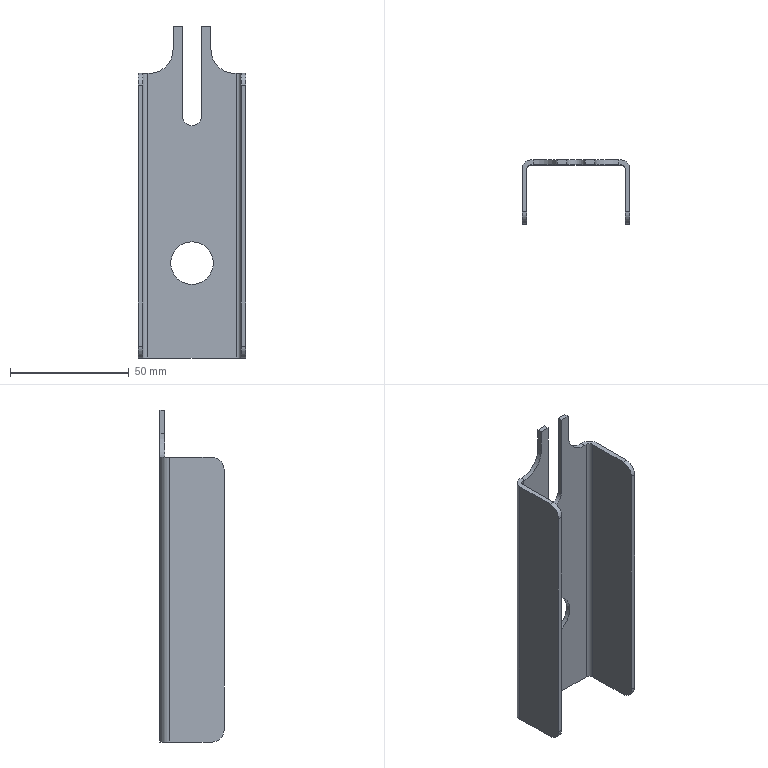Part | NX | features BREP 1 | 1 solid | 29 faces | box 45.5 x 27 x 140 mm | volume 21818 mm3 | plane 17 | cylinder 12 | commonest cylinder face diameters 10 x4 8 x3 4 x2 20 x2 18 x1
STEP:
#1=CARTESIAN_POINT('',(4.,0.,140.));
#2=VERTEX_POINT('',#1);
#3=CARTESIAN_POINT('',(4.,0.,102.));
#4=VERTEX_POINT('',#3);
#5=CARTESIAN_POINT('',(4.,0.,140.));
#6=DIRECTION('',(0.,0.,-1.));
#7=VECTOR('',#6,1000.);
#8=LINE('',#5,#7);
#9=EDGE_CURVE('',#2,#4,#8,.T.);
#10=ORIENTED_EDGE('',*,*,#9,.T.);
#11=CARTESIAN_POINT('',(-4.,0.,102.));
#12=VERTEX_POINT('',#11);
#13=CARTESIAN_POINT('',(0.,0.,102.));
#14=DIRECTION('',(0.,1.,0.));
#15=DIRECTION('',(0.,0.,1.));
#16=AXIS2_PLACEMENT_3D('',#13,#14,#15);
#17=CIRCLE('',#16,4.);
#18=EDGE_CURVE('',#4,#12,#17,.T.);
#19=ORIENTED_EDGE('',*,*,#18,.T.);
#20=CARTESIAN_POINT('',(-4.,0.,140.));
#21=VERTEX_POINT('',#20);
#22=CARTESIAN_POINT('',(-4.,0.,140.));
#23=DIRECTION('',(0.,0.,1.));
#24=VECTOR('',#23,1000.);
#25=LINE('',#22,#24);
#26=EDGE_CURVE('',#12,#21,#25,.T.);
#27=ORIENTED_EDGE('',*,*,#26,.T.);
#28=CARTESIAN_POINT('',(-8.,0.,140.));
#29=VERTEX_POINT('',#28);
#30=CARTESIAN_POINT('',(-20.75,0.,140.));
#31=DIRECTION('',(-1.,0.,0.));
#32=VECTOR('',#31,1000.);
#33=LINE('',#30,#32);
#34=EDGE_CURVE('',#21,#29,#33,.T.);
#35=ORIENTED_EDGE('',*,*,#34,.T.);
#36=CARTESIAN_POINT('',(-8.,0.,130.));
#37=VERTEX_POINT('',#36);
#38=CARTESIAN_POINT('',(-8.,0.,140.));
#39=DIRECTION('',(0.,0.,-1.));
#40=VECTOR('',#39,1000.);
#41=LINE('',#38,#40);
#42=EDGE_CURVE('',#29,#37,#41,.T.);
#43=ORIENTED_EDGE('',*,*,#42,.T.);
#44=CARTESIAN_POINT('',(-18.,0.,120.));
#45=VERTEX_POINT('',#44);
#46=CARTESIAN_POINT('',(-18.,0.,130.));
#47=DIRECTION('',(0.,1.,0.));
#48=DIRECTION('',(0.,0.,-1.));
#49=AXIS2_PLACEMENT_3D('',#46,#47,#48);
#50=CIRCLE('',#49,10.);
#51=EDGE_CURVE('',#37,#45,#50,.T.);
#52=ORIENTED_EDGE('',*,*,#51,.T.);
#53=CARTESIAN_POINT('',(-18.75,0.,120.));
#54=VERTEX_POINT('',#53);
#55=CARTESIAN_POINT('',(-8.,0.,120.));
#56=DIRECTION('',(-1.,0.,0.));
#57=VECTOR('',#56,1000.);
#58=LINE('',#55,#57);
#59=EDGE_CURVE('',#45,#54,#58,.T.);
#60=ORIENTED_EDGE('',*,*,#59,.T.);
#61=CARTESIAN_POINT('',(-18.75,0.,0.));
#62=VERTEX_POINT('',#61);
#63=CARTESIAN_POINT('',(-18.75,0.,140.));
#64=DIRECTION('',(0.,0.,-1.));
#65=VECTOR('',#64,1000.);
#66=LINE('',#63,#65);
#67=EDGE_CURVE('',#54,#62,#66,.T.);
#68=ORIENTED_EDGE('',*,*,#67,.T.);
#69=CARTESIAN_POINT('',(18.75,0.,0.));
#70=VERTEX_POINT('',#69);
#71=CARTESIAN_POINT('',(-20.75,0.,0.));
#72=DIRECTION('',(1.,0.,0.));
#73=VECTOR('',#72,1000.);
#74=LINE('',#71,#73);
#75=EDGE_CURVE('',#62,#70,#74,.T.);
#76=ORIENTED_EDGE('',*,*,#75,.T.);
#77=CARTESIAN_POINT('',(18.75,0.,120.));
#78=VERTEX_POINT('',#77);
#79=CARTESIAN_POINT('',(18.75,0.,140.));
#80=DIRECTION('',(0.,0.,1.));
#81=VECTOR('',#80,1000.);
#82=LINE('',#79,#81);
#83=EDGE_CURVE('',#70,#78,#82,.T.);
#84=ORIENTED_EDGE('',*,*,#83,.T.);
#85=CARTESIAN_POINT('',(18.,0.,120.));
#86=VERTEX_POINT('',#85);
#87=CARTESIAN_POINT('',(8.,0.,120.));
#88=DIRECTION('',(1.,0.,0.));
#89=VECTOR('',#88,1000.);
#90=LINE('',#87,#89);
#91=EDGE_CURVE('',#86,#78,#90,.T.);
#92=ORIENTED_EDGE('',*,*,#91,.F.);
#93=CARTESIAN_POINT('',(8.,0.,130.));
#94=VERTEX_POINT('',#93);
#95=CARTESIAN_POINT('',(18.,0.,130.));
#96=DIRECTION('',(0.,1.,0.));
#97=DIRECTION('',(0.,0.,-1.));
#98=AXIS2_PLACEMENT_3D('',#95,#96,#97);
#99=CIRCLE('',#98,10.);
#100=EDGE_CURVE('',#86,#94,#99,.T.);
#101=ORIENTED_EDGE('',*,*,#100,.T.);
#102=CARTESIAN_POINT('',(8.,0.,140.));
#103=VERTEX_POINT('',#102);
#104=CARTESIAN_POINT('',(8.,0.,140.));
#105=DIRECTION('',(0.,0.,1.));
#106=VECTOR('',#105,1000.);
#107=LINE('',#104,#106);
#108=EDGE_CURVE('',#94,#103,#107,.T.);
#109=ORIENTED_EDGE('',*,*,#108,.T.);
#110=CARTESIAN_POINT('',(-20.75,0.,140.));
#111=DIRECTION('',(-1.,0.,0.));
#112=VECTOR('',#111,1000.);
#113=LINE('',#110,#112);
#114=EDGE_CURVE('',#103,#2,#113,.T.);
#115=ORIENTED_EDGE('',*,*,#114,.T.);
#116=EDGE_LOOP('',(#10,#19,#27,#35,#43,#52,#60,#68,#76,#84,#92,#101,#109,#115));
#117=FACE_BOUND('',#116,.T.);
#118=CARTESIAN_POINT('',(0.,0.,49.));
#119=VERTEX_POINT('',#118);
#120=CARTESIAN_POINT('',(0.,0.,40.));
#121=DIRECTION('',(0.,1.,0.));
#122=DIRECTION('',(0.,0.,1.));
#123=AXIS2_PLACEMENT_3D('',#120,#121,#122);
#124=CIRCLE('',#123,9.);
#125=EDGE_CURVE('',#119,#119,#124,.T.);
#126=ORIENTED_EDGE('',*,*,#125,.T.);
#127=EDGE_LOOP('',(#126));
#128=FACE_BOUND('',#127,.T.);
#129=CARTESIAN_POINT('',(-20.75,0.,140.));
#130=DIRECTION('',(0.,-1.,0.));
#131=DIRECTION('',(0.,0.,1.));
#132=AXIS2_PLACEMENT_3D('',#129,#130,#131);
#133=PLANE('',#132);
#134=ADVANCED_FACE('',(#117,#128),#133,.T.);
#135=CARTESIAN_POINT('',(4.,2.,102.));
#136=VERTEX_POINT('',#135);
#137=CARTESIAN_POINT('',(4.,-8.,102.));
#138=DIRECTION('',(0.,-1.,0.));
#139=VECTOR('',#138,1000.);
#140=LINE('',#137,#139);
#141=EDGE_CURVE('',#136,#4,#140,.T.);
#142=ORIENTED_EDGE('',*,*,#141,.F.);
#143=CARTESIAN_POINT('',(-4.,2.,102.));
#144=VERTEX_POINT('',#143);
#145=CARTESIAN_POINT('',(0.,2.,102.));
#146=DIRECTION('',(0.,-1.,0.));
#147=DIRECTION('',(0.,0.,1.));
#148=AXIS2_PLACEMENT_3D('',#145,#146,#147);
#149=CIRCLE('',#148,4.);
#150=EDGE_CURVE('',#144,#136,#149,.T.);
#151=ORIENTED_EDGE('',*,*,#150,.F.);
#152=CARTESIAN_POINT('',(-4.,-8.,102.));
#153=DIRECTION('',(0.,1.,0.));
#154=VECTOR('',#153,1000.);
#155=LINE('',#152,#154);
#156=EDGE_CURVE('',#12,#144,#155,.T.);
#157=ORIENTED_EDGE('',*,*,#156,.F.);
#158=ORIENTED_EDGE('',*,*,#18,.F.);
#159=EDGE_LOOP('',(#142,#151,#157,#158));
#160=FACE_BOUND('',#159,.T.);
#161=CARTESIAN_POINT('',(0.,-8.,102.));
#162=DIRECTION('',(0.,1.,0.));
#163=DIRECTION('',(0.,0.,-1.));
#164=AXIS2_PLACEMENT_3D('',#161,#162,#163);
#165=CYLINDRICAL_SURFACE('',#164,4.);
#166=ADVANCED_FACE('',(#160),#165,.F.);
#167=CARTESIAN_POINT('',(4.,2.,140.));
#168=VERTEX_POINT('',#167);
#169=CARTESIAN_POINT('',(4.,-8.,140.));
#170=DIRECTION('',(0.,-1.,0.));
#171=VECTOR('',#170,1000.);
#172=LINE('',#169,#171);
#173=EDGE_CURVE('',#168,#2,#172,.T.);
#174=ORIENTED_EDGE('',*,*,#173,.F.);
#175=CARTESIAN_POINT('',(4.,2.,140.));
#176=DIRECTION('',(0.,0.,1.));
#177=VECTOR('',#176,1000.);
#178=LINE('',#175,#177);
#179=EDGE_CURVE('',#136,#168,#178,.T.);
#180=ORIENTED_EDGE('',*,*,#179,.F.);
#181=ORIENTED_EDGE('',*,*,#141,.T.);
#182=ORIENTED_EDGE('',*,*,#9,.F.);
#183=EDGE_LOOP('',(#174,#180,#181,#182));
#184=FACE_BOUND('',#183,.T.);
#185=CARTESIAN_POINT('',(4.,-8.,140.));
#186=DIRECTION('',(1.,0.,0.));
#187=DIRECTION('',(0.,0.,1.));
#188=AXIS2_PLACEMENT_3D('',#185,#186,#187);
#189=PLANE('',#188);
#190=ADVANCED_FACE('',(#184),#189,.F.);
#191=CARTESIAN_POINT('',(8.,2.,140.));
#192=VERTEX_POINT('',#191);
#193=CARTESIAN_POINT('',(8.,-2.,140.));
#194=DIRECTION('',(0.,1.,0.));
#195=VECTOR('',#194,1000.);
#196=LINE('',#193,#195);
#197=EDGE_CURVE('',#103,#192,#196,.T.);
#198=ORIENTED_EDGE('',*,*,#197,.T.);
#199=CARTESIAN_POINT('',(22.75,2.,140.));
#200=DIRECTION('',(-1.,0.,0.));
#201=VECTOR('',#200,1000.);
#202=LINE('',#199,#201);
#203=EDGE_CURVE('',#192,#168,#202,.T.);
#204=ORIENTED_EDGE('',*,*,#203,.T.);
#205=ORIENTED_EDGE('',*,*,#173,.T.);
#206=ORIENTED_EDGE('',*,*,#114,.F.);
#207=EDGE_LOOP('',(#198,#204,#205,#206));
#208=FACE_BOUND('',#207,.T.);
#209=CARTESIAN_POINT('',(22.75,-2.,140.));
#210=DIRECTION('',(0.,0.,1.));
#211=DIRECTION('',(-1.,0.,0.));
#212=AXIS2_PLACEMENT_3D('',#209,#210,#211);
#213=PLANE('',#212);
#214=ADVANCED_FACE('',(#208),#213,.T.);
#215=CARTESIAN_POINT('',(8.,2.,130.));
#216=VERTEX_POINT('',#215);
#217=CARTESIAN_POINT('',(8.,2.,120.));
#218=DIRECTION('',(0.,0.,1.));
#219=VECTOR('',#218,1000.);
#220=LINE('',#217,#219);
#221=EDGE_CURVE('',#216,#192,#220,.T.);
#222=ORIENTED_EDGE('',*,*,#221,.T.);
#223=ORIENTED_EDGE('',*,*,#197,.F.);
#224=ORIENTED_EDGE('',*,*,#108,.F.);
#225=CARTESIAN_POINT('',(8.,-25.,130.));
#226=DIRECTION('',(0.,1.,0.));
#227=VECTOR('',#226,1000.);
#228=LINE('',#225,#227);
#229=EDGE_CURVE('',#94,#216,#228,.T.);
#230=ORIENTED_EDGE('',*,*,#229,.T.);
#231=EDGE_LOOP('',(#222,#223,#224,#230));
#232=FACE_BOUND('',#231,.T.);
#233=CARTESIAN_POINT('',(8.,-25.,120.));
#234=DIRECTION('',(1.,0.,0.));
#235=DIRECTION('',(0.,0.,1.));
#236=AXIS2_PLACEMENT_3D('',#233,#234,#235);
#237=PLANE('',#236);
#238=ADVANCED_FACE('',(#232),#237,.T.);
#239=CARTESIAN_POINT('',(18.,2.,120.));
#240=VERTEX_POINT('',#239);
#241=CARTESIAN_POINT('',(18.,-25.,120.));
#242=DIRECTION('',(0.,-1.,0.));
#243=VECTOR('',#242,1000.);
#244=LINE('',#241,#243);
#245=EDGE_CURVE('',#240,#86,#244,.T.);
#246=ORIENTED_EDGE('',*,*,#245,.F.);
#247=CARTESIAN_POINT('',(18.,2.,130.));
#248=DIRECTION('',(0.,-1.,0.));
#249=DIRECTION('',(0.,0.,-1.));
#250=AXIS2_PLACEMENT_3D('',#247,#248,#249);
#251=CIRCLE('',#250,10.);
#252=EDGE_CURVE('',#216,#240,#251,.T.);
#253=ORIENTED_EDGE('',*,*,#252,.F.);
#254=ORIENTED_EDGE('',*,*,#229,.F.);
#255=ORIENTED_EDGE('',*,*,#100,.F.);
#256=EDGE_LOOP('',(#246,#253,#254,#255));
#257=FACE_BOUND('',#256,.T.);
#258=CARTESIAN_POINT('',(18.,-25.,130.));
#259=DIRECTION('',(0.,-1.,0.));
#260=DIRECTION('',(0.,0.,1.));
#261=AXIS2_PLACEMENT_3D('',#258,#259,#260);
#262=CYLINDRICAL_SURFACE('',#261,10.);
#263=ADVANCED_FACE('',(#257),#262,.F.);
#264=CARTESIAN_POINT('',(20.75,-2.,120.));
#265=VERTEX_POINT('',#264);
#266=CARTESIAN_POINT('',(18.75,-2.,120.));
#267=DIRECTION('',(0.,0.,-1.));
#268=DIRECTION('',(-1.,0.,0.));
#269=AXIS2_PLACEMENT_3D('',#266,#267,#268);
#270=CIRCLE('',#269,2.);
#271=EDGE_CURVE('',#78,#265,#270,.T.);
#272=ORIENTED_EDGE('',*,*,#271,.F.);
#273=ORIENTED_EDGE('',*,*,#83,.F.);
#274=CARTESIAN_POINT('',(20.75,-2.,0.));
#275=VERTEX_POINT('',#274);
#276=CARTESIAN_POINT('',(18.75,-2.,0.));
#277=DIRECTION('',(0.,0.,1.));
#278=DIRECTION('',(-1.,0.,0.));
#279=AXIS2_PLACEMENT_3D('',#276,#277,#278);
#280=CIRCLE('',#279,2.);
#281=EDGE_CURVE('',#275,#70,#280,.T.);
#282=ORIENTED_EDGE('',*,*,#281,.F.);
#283=CARTESIAN_POINT('',(20.75,-2.,140.));
#284=DIRECTION('',(0.,0.,-1.));
#285=VECTOR('',#284,1000.);
#286=LINE('',#283,#285);
#287=EDGE_CURVE('',#265,#275,#286,.T.);
#288=ORIENTED_EDGE('',*,*,#287,.F.);
#289=EDGE_LOOP('',(#272,#273,#282,#288));
#290=FACE_BOUND('',#289,.T.);
#291=CARTESIAN_POINT('',(18.75,-2.,140.));
#292=DIRECTION('',(0.,0.,-1.));
#293=DIRECTION('',(1.,0.,0.));
#294=AXIS2_PLACEMENT_3D('',#291,#292,#293);
#295=CYLINDRICAL_SURFACE('',#294,2.);
#296=ADVANCED_FACE('',(#290),#295,.F.);
#297=CARTESIAN_POINT('',(-18.75,2.,0.));
#298=VERTEX_POINT('',#297);
#299=CARTESIAN_POINT('',(18.75,2.,0.));
#300=VERTEX_POINT('',#299);
#301=CARTESIAN_POINT('',(-22.75,2.,0.));
#302=DIRECTION('',(1.,0.,0.));
#303=VECTOR('',#302,1000.);
#304=LINE('',#301,#303);
#305=EDGE_CURVE('',#298,#300,#304,.T.);
#306=ORIENTED_EDGE('',*,*,#305,.T.);
#307=CARTESIAN_POINT('',(22.75,-2.,0.));
#308=VERTEX_POINT('',#307);
#309=CARTESIAN_POINT('',(18.75,-2.,0.));
#310=DIRECTION('',(0.,0.,-1.));
#311=DIRECTION('',(-1.,0.,0.));
#312=AXIS2_PLACEMENT_3D('',#309,#310,#311);
#313=CIRCLE('',#312,4.);
#314=EDGE_CURVE('',#300,#308,#313,.T.);
#315=ORIENTED_EDGE('',*,*,#314,.T.);
#316=CARTESIAN_POINT('',(22.75,-20.,0.));
#317=VERTEX_POINT('',#316);
#318=CARTESIAN_POINT('',(22.75,0.,0.));
#319=DIRECTION('',(0.,-1.,0.));
#320=VECTOR('',#319,1000.);
#321=LINE('',#318,#320);
#322=EDGE_CURVE('',#308,#317,#321,.T.);
#323=ORIENTED_EDGE('',*,*,#322,.T.);
#324=CARTESIAN_POINT('',(20.75,-20.,0.));
#325=VERTEX_POINT('',#324);
#326=CARTESIAN_POINT('',(18.75,-20.,0.));
#327=DIRECTION('',(1.,0.,0.));
#328=VECTOR('',#327,1000.);
#329=LINE('',#326,#328);
#330=EDGE_CURVE('',#325,#317,#329,.T.);
#331=ORIENTED_EDGE('',*,*,#330,.F.);
#332=CARTESIAN_POINT('',(20.75,0.,0.));
#333=DIRECTION('',(0.,-1.,0.));
#334=VECTOR('',#333,1000.);
#335=LINE('',#332,#334);
#336=EDGE_CURVE('',#275,#325,#335,.T.);
#337=ORIENTED_EDGE('',*,*,#336,.F.);
#338=ORIENTED_EDGE('',*,*,#281,.T.);
#339=ORIENTED_EDGE('',*,*,#75,.F.);
#340=CARTESIAN_POINT('',(-20.75,-2.,0.));
#341=VERTEX_POINT('',#340);
#342=CARTESIAN_POINT('',(-18.75,-2.,0.));
#343=DIRECTION('',(0.,0.,1.));
#344=DIRECTION('',(-1.,0.,0.));
#345=AXIS2_PLACEMENT_3D('',#342,#343,#344);
#346=CIRCLE('',#345,2.);
#347=EDGE_CURVE('',#62,#341,#346,.T.);
#348=ORIENTED_EDGE('',*,*,#347,.T.);
#349=CARTESIAN_POINT('',(-20.75,-20.,0.));
#350=VERTEX_POINT('',#349);
#351=CARTESIAN_POINT('',(-20.75,0.,0.));
#352=DIRECTION('',(0.,1.,0.));
#353=VECTOR('',#352,1000.);
#354=LINE('',#351,#353);
#355=EDGE_CURVE('',#350,#341,#354,.T.);
#356=ORIENTED_EDGE('',*,*,#355,.F.);
#357=CARTESIAN_POINT('',(-22.75,-20.,0.));
#358=VERTEX_POINT('',#357);
#359=CARTESIAN_POINT('',(-18.75,-20.,0.));
#360=DIRECTION('',(-1.,0.,0.));
#361=VECTOR('',#360,1000.);
#362=LINE('',#359,#361);
#363=EDGE_CURVE('',#350,#358,#362,.T.);
#364=ORIENTED_EDGE('',*,*,#363,.T.);
#365=CARTESIAN_POINT('',(-22.75,-2.,0.));
#366=VERTEX_POINT('',#365);
#367=CARTESIAN_POINT('',(-22.75,-2.,0.));
#368=DIRECTION('',(0.,1.,0.));
#369=VECTOR('',#368,1000.);
#370=LINE('',#367,#369);
#371=EDGE_CURVE('',#358,#366,#370,.T.);
#372=ORIENTED_EDGE('',*,*,#371,.T.);
#373=CARTESIAN_POINT('',(-18.75,-2.,0.));
#374=DIRECTION('',(0.,0.,-1.));
#375=DIRECTION('',(-1.,0.,0.));
#376=AXIS2_PLACEMENT_3D('',#373,#374,#375);
#377=CIRCLE('',#376,4.);
#378=EDGE_CURVE('',#366,#298,#377,.T.);
#379=ORIENTED_EDGE('',*,*,#378,.T.);
#380=EDGE_LOOP('',(#306,#315,#323,#331,#337,#338,#339,#348,#356,#364,#372,#379));
#381=FACE_BOUND('',#380,.T.);
#382=CARTESIAN_POINT('',(-22.75,-2.,0.));
#383=DIRECTION('',(0.,0.,-1.));
#384=DIRECTION('',(1.,0.,0.));
#385=AXIS2_PLACEMENT_3D('',#382,#383,#384);
#386=PLANE('',#385);
#387=ADVANCED_FACE('',(#381),#386,.T.);
#388=CARTESIAN_POINT('',(-20.75,-2.,120.));
#389=VERTEX_POINT('',#388);
#390=CARTESIAN_POINT('',(-20.75,-2.,140.));
#391=DIRECTION('',(0.,0.,1.));
#392=VECTOR('',#391,1000.);
#393=LINE('',#390,#392);
#394=EDGE_CURVE('',#341,#389,#393,.T.);
#395=ORIENTED_EDGE('',*,*,#394,.F.);
#396=ORIENTED_EDGE('',*,*,#347,.F.);
#397=ORIENTED_EDGE('',*,*,#67,.F.);
#398=CARTESIAN_POINT('',(-18.75,-2.,120.));
#399=DIRECTION('',(0.,0.,-1.));
#400=DIRECTION('',(-1.,0.,0.));
#401=AXIS2_PLACEMENT_3D('',#398,#399,#400);
#402=CIRCLE('',#401,2.);
#403=EDGE_CURVE('',#389,#54,#402,.T.);
#404=ORIENTED_EDGE('',*,*,#403,.F.);
#405=EDGE_LOOP('',(#395,#396,#397,#404));
#406=FACE_BOUND('',#405,.T.);
#407=CARTESIAN_POINT('',(-18.75,-2.,140.));
#408=DIRECTION('',(0.,0.,-1.));
#409=DIRECTION('',(1.,0.,0.));
#410=AXIS2_PLACEMENT_3D('',#407,#408,#409);
#411=CYLINDRICAL_SURFACE('',#410,2.);
#412=ADVANCED_FACE('',(#406),#411,.F.);
#413=CARTESIAN_POINT('',(-8.,2.,130.));
#414=VERTEX_POINT('',#413);
#415=CARTESIAN_POINT('',(-8.,-25.,130.));
#416=DIRECTION('',(0.,-1.,0.));
#417=VECTOR('',#416,1000.);
#418=LINE('',#415,#417);
#419=EDGE_CURVE('',#414,#37,#418,.T.);
#420=ORIENTED_EDGE('',*,*,#419,.F.);
#421=CARTESIAN_POINT('',(-18.,2.,120.));
#422=VERTEX_POINT('',#421);
#423=CARTESIAN_POINT('',(-18.,2.,130.));
#424=DIRECTION('',(0.,-1.,0.));
#425=DIRECTION('',(0.,0.,-1.));
#426=AXIS2_PLACEMENT_3D('',#423,#424,#425);
#427=CIRCLE('',#426,10.);
#428=EDGE_CURVE('',#422,#414,#427,.T.);
#429=ORIENTED_EDGE('',*,*,#428,.F.);
#430=CARTESIAN_POINT('',(-18.,-25.,120.));
#431=DIRECTION('',(0.,1.,0.));
#432=VECTOR('',#431,1000.);
#433=LINE('',#430,#432);
#434=EDGE_CURVE('',#45,#422,#433,.T.);
#435=ORIENTED_EDGE('',*,*,#434,.F.);
#436=ORIENTED_EDGE('',*,*,#51,.F.);
#437=EDGE_LOOP('',(#420,#429,#435,#436));
#438=FACE_BOUND('',#437,.T.);
#439=CARTESIAN_POINT('',(-18.,-25.,130.));
#440=DIRECTION('',(0.,-1.,0.));
#441=DIRECTION('',(0.,0.,1.));
#442=AXIS2_PLACEMENT_3D('',#439,#440,#441);
#443=CYLINDRICAL_SURFACE('',#442,10.);
#444=ADVANCED_FACE('',(#438),#443,.F.);
#445=ORIENTED_EDGE('',*,*,#419,.T.);
#446=ORIENTED_EDGE('',*,*,#42,.F.);
#447=CARTESIAN_POINT('',(-8.,2.,140.));
#448=VERTEX_POINT('',#447);
#449=CARTESIAN_POINT('',(-8.,-25.,140.));
#450=DIRECTION('',(0.,-1.,0.));
#451=VECTOR('',#450,1000.);
#452=LINE('',#449,#451);
#453=EDGE_CURVE('',#448,#29,#452,.T.);
#454=ORIENTED_EDGE('',*,*,#453,.F.);
#455=CARTESIAN_POINT('',(-8.,2.,120.));
#456=DIRECTION('',(0.,0.,1.));
#457=VECTOR('',#456,1000.);
#458=LINE('',#455,#457);
#459=EDGE_CURVE('',#414,#448,#458,.T.);
#460=ORIENTED_EDGE('',*,*,#459,.F.);
#461=EDGE_LOOP('',(#445,#446,#454,#460));
#462=FACE_BOUND('',#461,.T.);
#463=CARTESIAN_POINT('',(-8.,-25.,120.));
#464=DIRECTION('',(1.,0.,0.));
#465=DIRECTION('',(0.,0.,1.));
#466=AXIS2_PLACEMENT_3D('',#463,#464,#465);
#467=PLANE('',#466);
#468=ADVANCED_FACE('',(#462),#467,.F.);
#469=ORIENTED_EDGE('',*,*,#453,.T.);
#470=ORIENTED_EDGE('',*,*,#34,.F.);
#471=CARTESIAN_POINT('',(-4.,2.,140.));
#472=VERTEX_POINT('',#471);
#473=CARTESIAN_POINT('',(-4.,-2.,140.));
#474=DIRECTION('',(0.,1.,0.));
#475=VECTOR('',#474,1000.);
#476=LINE('',#473,#475);
#477=EDGE_CURVE('',#21,#472,#476,.T.);
#478=ORIENTED_EDGE('',*,*,#477,.T.);
#479=CARTESIAN_POINT('',(22.75,2.,140.));
#480=DIRECTION('',(-1.,0.,0.));
#481=VECTOR('',#480,1000.);
#482=LINE('',#479,#481);
#483=EDGE_CURVE('',#472,#448,#482,.T.);
#484=ORIENTED_EDGE('',*,*,#483,.T.);
#485=EDGE_LOOP('',(#469,#470,#478,#484));
#486=FACE_BOUND('',#485,.T.);
#487=CARTESIAN_POINT('',(22.75,-2.,140.));
#488=DIRECTION('',(0.,0.,1.));
#489=DIRECTION('',(-1.,0.,0.));
#490=AXIS2_PLACEMENT_3D('',#487,#488,#489);
#491=PLANE('',#490);
#492=ADVANCED_FACE('',(#486),#491,.T.);
#493=ORIENTED_EDGE('',*,*,#156,.T.);
#494=CARTESIAN_POINT('',(-4.,2.,140.));
#495=DIRECTION('',(0.,0.,-1.));
#496=VECTOR('',#495,1000.);
#497=LINE('',#494,#496);
#498=EDGE_CURVE('',#472,#144,#497,.T.);
#499=ORIENTED_EDGE('',*,*,#498,.F.);
#500=ORIENTED_EDGE('',*,*,#477,.F.);
#501=ORIENTED_EDGE('',*,*,#26,.F.);
#502=EDGE_LOOP('',(#493,#499,#500,#501));
#503=FACE_BOUND('',#502,.T.);
#504=CARTESIAN_POINT('',(-4.,-8.,140.));
#505=DIRECTION('',(-1.,0.,0.));
#506=DIRECTION('',(0.,0.,-1.));
#507=AXIS2_PLACEMENT_3D('',#504,#505,#506);
#508=PLANE('',#507);
#509=ADVANCED_FACE('',(#503),#508,.F.);
#510=ORIENTED_EDGE('',*,*,#125,.F.);
#511=EDGE_LOOP('',(#510));
#512=FACE_BOUND('',#511,.T.);
#513=CARTESIAN_POINT('',(0.,2.,49.));
#514=VERTEX_POINT('',#513);
#515=CARTESIAN_POINT('',(0.,2.,40.));
#516=DIRECTION('',(0.,-1.,0.));
#517=DIRECTION('',(0.,0.,1.));
#518=AXIS2_PLACEMENT_3D('',#515,#516,#517);
#519=CIRCLE('',#518,9.);
#520=EDGE_CURVE('',#514,#514,#519,.T.);
#521=ORIENTED_EDGE('',*,*,#520,.F.);
#522=EDGE_LOOP('',(#521));
#523=FACE_BOUND('',#522,.T.);
#524=CARTESIAN_POINT('',(0.,-8.,40.));
#525=DIRECTION('',(0.,1.,0.));
#526=DIRECTION('',(0.,0.,-1.));
#527=AXIS2_PLACEMENT_3D('',#524,#525,#526);
#528=CYLINDRICAL_SURFACE('',#527,9.);
#529=ADVANCED_FACE('',(#512,#523),#528,.F.);
#530=ORIENTED_EDGE('',*,*,#498,.T.);
#531=ORIENTED_EDGE('',*,*,#150,.T.);
#532=ORIENTED_EDGE('',*,*,#179,.T.);
#533=ORIENTED_EDGE('',*,*,#203,.F.);
#534=ORIENTED_EDGE('',*,*,#221,.F.);
#535=ORIENTED_EDGE('',*,*,#252,.T.);
#536=CARTESIAN_POINT('',(18.75,2.,120.));
#537=VERTEX_POINT('',#536);
#538=CARTESIAN_POINT('',(-20.75,2.,120.));
#539=DIRECTION('',(-1.,0.,0.));
#540=VECTOR('',#539,1000.);
#541=LINE('',#538,#540);
#542=EDGE_CURVE('',#537,#240,#541,.T.);
#543=ORIENTED_EDGE('',*,*,#542,.F.);
#544=CARTESIAN_POINT('',(18.75,2.,140.));
#545=DIRECTION('',(0.,0.,1.));
#546=VECTOR('',#545,1000.);
#547=LINE('',#544,#546);
#548=EDGE_CURVE('',#300,#537,#547,.T.);
#549=ORIENTED_EDGE('',*,*,#548,.F.);
#550=ORIENTED_EDGE('',*,*,#305,.F.);
#551=CARTESIAN_POINT('',(-18.75,2.,120.));
#552=VERTEX_POINT('',#551);
#553=CARTESIAN_POINT('',(-18.75,2.,140.));
#554=DIRECTION('',(0.,0.,-1.));
#555=VECTOR('',#554,1000.);
#556=LINE('',#553,#555);
#557=EDGE_CURVE('',#552,#298,#556,.T.);
#558=ORIENTED_EDGE('',*,*,#557,.F.);
#559=CARTESIAN_POINT('',(-20.75,2.,120.));
#560=DIRECTION('',(-1.,0.,0.));
#561=VECTOR('',#560,1000.);
#562=LINE('',#559,#561);
#563=EDGE_CURVE('',#422,#552,#562,.T.);
#564=ORIENTED_EDGE('',*,*,#563,.F.);
#565=ORIENTED_EDGE('',*,*,#428,.T.);
#566=ORIENTED_EDGE('',*,*,#459,.T.);
#567=ORIENTED_EDGE('',*,*,#483,.F.);
#568=EDGE_LOOP('',(#530,#531,#532,#533,#534,#535,#543,#549,#550,#558,#564,#565,#566,#567));
#569=FACE_BOUND('',#568,.T.);
#570=ORIENTED_EDGE('',*,*,#520,.T.);
#571=EDGE_LOOP('',(#570));
#572=FACE_BOUND('',#571,.T.);
#573=CARTESIAN_POINT('',(-20.75,2.,140.));
#574=DIRECTION('',(0.,-1.,0.));
#575=DIRECTION('',(0.,0.,1.));
#576=AXIS2_PLACEMENT_3D('',#573,#574,#575);
#577=PLANE('',#576);
#578=ADVANCED_FACE('',(#569,#572),#577,.F.);
#579=ORIENTED_EDGE('',*,*,#91,.T.);
#580=ORIENTED_EDGE('',*,*,#271,.T.);
#581=CARTESIAN_POINT('',(20.75,-20.,120.));
#582=VERTEX_POINT('',#581);
#583=CARTESIAN_POINT('',(20.75,-25.,120.));
#584=DIRECTION('',(0.,-1.,0.));
#585=VECTOR('',#584,1000.);
#586=LINE('',#583,#585);
#587=EDGE_CURVE('',#265,#582,#586,.T.);
#588=ORIENTED_EDGE('',*,*,#587,.T.);
#589=CARTESIAN_POINT('',(22.75,-20.,120.));
#590=VERTEX_POINT('',#589);
#591=CARTESIAN_POINT('',(8.,-20.,120.));
#592=DIRECTION('',(1.,0.,0.));
#593=VECTOR('',#592,1000.);
#594=LINE('',#591,#593);
#595=EDGE_CURVE('',#582,#590,#594,.T.);
#596=ORIENTED_EDGE('',*,*,#595,.T.);
#597=CARTESIAN_POINT('',(22.75,-2.,120.));
#598=VERTEX_POINT('',#597);
#599=CARTESIAN_POINT('',(22.75,-25.,120.));
#600=DIRECTION('',(0.,1.,0.));
#601=VECTOR('',#600,1000.);
#602=LINE('',#599,#601);
#603=EDGE_CURVE('',#590,#598,#602,.T.);
#604=ORIENTED_EDGE('',*,*,#603,.T.);
#605=CARTESIAN_POINT('',(18.75,-2.,120.));
#606=DIRECTION('',(0.,0.,1.));
#607=DIRECTION('',(-1.,0.,0.));
#608=AXIS2_PLACEMENT_3D('',#605,#606,#607);
#609=CIRCLE('',#608,4.);
#610=EDGE_CURVE('',#598,#537,#609,.T.);
#611=ORIENTED_EDGE('',*,*,#610,.T.);
#612=ORIENTED_EDGE('',*,*,#542,.T.);
#613=ORIENTED_EDGE('',*,*,#245,.T.);
#614=EDGE_LOOP('',(#579,#580,#588,#596,#604,#611,#612,#613));
#615=FACE_BOUND('',#614,.T.);
#616=CARTESIAN_POINT('',(8.,-25.,120.));
#617=DIRECTION('',(0.,0.,1.));
#618=DIRECTION('',(-1.,0.,0.));
#619=AXIS2_PLACEMENT_3D('',#616,#617,#618);
#620=PLANE('',#619);
#621=ADVANCED_FACE('',(#615),#620,.T.);
#622=ORIENTED_EDGE('',*,*,#336,.T.);
#623=CARTESIAN_POINT('',(20.75,-25.,5.));
#624=VERTEX_POINT('',#623);
#625=CARTESIAN_POINT('',(20.75,-20.,5.));
#626=DIRECTION('',(-1.,0.,0.));
#627=DIRECTION('',(0.,0.,1.));
#628=AXIS2_PLACEMENT_3D('',#625,#626,#627);
#629=CIRCLE('',#628,5.);
#630=EDGE_CURVE('',#325,#624,#629,.T.);
#631=ORIENTED_EDGE('',*,*,#630,.T.);
#632=CARTESIAN_POINT('',(20.75,-25.,115.));
#633=VERTEX_POINT('',#632);
#634=CARTESIAN_POINT('',(20.75,-25.,140.));
#635=DIRECTION('',(0.,0.,1.));
#636=VECTOR('',#635,1000.);
#637=LINE('',#634,#636);
#638=EDGE_CURVE('',#624,#633,#637,.T.);
#639=ORIENTED_EDGE('',*,*,#638,.T.);
#640=CARTESIAN_POINT('',(20.75,-20.,115.));
#641=DIRECTION('',(-1.,0.,0.));
#642=DIRECTION('',(0.,0.,-1.));
#643=AXIS2_PLACEMENT_3D('',#640,#641,#642);
#644=CIRCLE('',#643,5.);
#645=EDGE_CURVE('',#633,#582,#644,.T.);
#646=ORIENTED_EDGE('',*,*,#645,.T.);
#647=ORIENTED_EDGE('',*,*,#587,.F.);
#648=ORIENTED_EDGE('',*,*,#287,.T.);
#649=EDGE_LOOP('',(#622,#631,#639,#646,#647,#648));
#650=FACE_BOUND('',#649,.T.);
#651=CARTESIAN_POINT('',(20.75,0.,140.));
#652=DIRECTION('',(-1.,0.,0.));
#653=DIRECTION('',(0.,0.,-1.));
#654=AXIS2_PLACEMENT_3D('',#651,#652,#653);
#655=PLANE('',#654);
#656=ADVANCED_FACE('',(#650),#655,.T.);
#657=CARTESIAN_POINT('',(-20.75,-20.,120.));
#658=VERTEX_POINT('',#657);
#659=CARTESIAN_POINT('',(-22.75,-20.,120.));
#660=VERTEX_POINT('',#659);
#661=CARTESIAN_POINT('',(-8.,-20.,120.));
#662=DIRECTION('',(-1.,0.,0.));
#663=VECTOR('',#662,1000.);
#664=LINE('',#661,#663);
#665=EDGE_CURVE('',#658,#660,#664,.T.);
#666=ORIENTED_EDGE('',*,*,#665,.F.);
#667=CARTESIAN_POINT('',(-20.75,-25.,120.));
#668=DIRECTION('',(0.,-1.,0.));
#669=VECTOR('',#668,1000.);
#670=LINE('',#667,#669);
#671=EDGE_CURVE('',#389,#658,#670,.T.);
#672=ORIENTED_EDGE('',*,*,#671,.F.);
#673=ORIENTED_EDGE('',*,*,#403,.T.);
#674=ORIENTED_EDGE('',*,*,#59,.F.);
#675=ORIENTED_EDGE('',*,*,#434,.T.);
#676=ORIENTED_EDGE('',*,*,#563,.T.);
#677=CARTESIAN_POINT('',(-22.75,-2.,120.));
#678=VERTEX_POINT('',#677);
#679=CARTESIAN_POINT('',(-18.75,-2.,120.));
#680=DIRECTION('',(0.,0.,-1.));
#681=DIRECTION('',(-1.,0.,0.));
#682=AXIS2_PLACEMENT_3D('',#679,#680,#681);
#683=CIRCLE('',#682,4.);
#684=EDGE_CURVE('',#678,#552,#683,.T.);
#685=ORIENTED_EDGE('',*,*,#684,.F.);
#686=CARTESIAN_POINT('',(-22.75,-25.,120.));
#687=DIRECTION('',(0.,1.,0.));
#688=VECTOR('',#687,1000.);
#689=LINE('',#686,#688);
#690=EDGE_CURVE('',#660,#678,#689,.T.);
#691=ORIENTED_EDGE('',*,*,#690,.F.);
#692=EDGE_LOOP('',(#666,#672,#673,#674,#675,#676,#685,#691));
#693=FACE_BOUND('',#692,.T.);
#694=CARTESIAN_POINT('',(-8.,-25.,120.));
#695=DIRECTION('',(0.,0.,-1.));
#696=DIRECTION('',(1.,0.,0.));
#697=AXIS2_PLACEMENT_3D('',#694,#695,#696);
#698=PLANE('',#697);
#699=ADVANCED_FACE('',(#693),#698,.F.);
#700=ORIENTED_EDGE('',*,*,#355,.T.);
#701=ORIENTED_EDGE('',*,*,#394,.T.);
#702=ORIENTED_EDGE('',*,*,#671,.T.);
#703=CARTESIAN_POINT('',(-20.75,-25.,115.));
#704=VERTEX_POINT('',#703);
#705=CARTESIAN_POINT('',(-20.75,-20.,115.));
#706=DIRECTION('',(1.,0.,0.));
#707=DIRECTION('',(0.,0.,-1.));
#708=AXIS2_PLACEMENT_3D('',#705,#706,#707);
#709=CIRCLE('',#708,5.);
#710=EDGE_CURVE('',#658,#704,#709,.T.);
#711=ORIENTED_EDGE('',*,*,#710,.T.);
#712=CARTESIAN_POINT('',(-20.75,-25.,5.));
#713=VERTEX_POINT('',#712);
#714=CARTESIAN_POINT('',(-20.75,-25.,140.));
#715=DIRECTION('',(0.,0.,-1.));
#716=VECTOR('',#715,1000.);
#717=LINE('',#714,#716);
#718=EDGE_CURVE('',#704,#713,#717,.T.);
#719=ORIENTED_EDGE('',*,*,#718,.T.);
#720=CARTESIAN_POINT('',(-20.75,-20.,5.));
#721=DIRECTION('',(1.,0.,0.));
#722=DIRECTION('',(0.,0.,1.));
#723=AXIS2_PLACEMENT_3D('',#720,#721,#722);
#724=CIRCLE('',#723,5.);
#725=EDGE_CURVE('',#713,#350,#724,.T.);
#726=ORIENTED_EDGE('',*,*,#725,.T.);
#727=EDGE_LOOP('',(#700,#701,#702,#711,#719,#726));
#728=FACE_BOUND('',#727,.T.);
#729=CARTESIAN_POINT('',(-20.75,0.,140.));
#730=DIRECTION('',(1.,0.,0.));
#731=DIRECTION('',(0.,0.,1.));
#732=AXIS2_PLACEMENT_3D('',#729,#730,#731);
#733=PLANE('',#732);
#734=ADVANCED_FACE('',(#728),#733,.T.);
#735=ORIENTED_EDGE('',*,*,#314,.F.);
#736=ORIENTED_EDGE('',*,*,#548,.T.);
#737=ORIENTED_EDGE('',*,*,#610,.F.);
#738=CARTESIAN_POINT('',(22.75,-2.,140.));
#739=DIRECTION('',(0.,0.,-1.));
#740=VECTOR('',#739,1000.);
#741=LINE('',#738,#740);
#742=EDGE_CURVE('',#598,#308,#741,.T.);
#743=ORIENTED_EDGE('',*,*,#742,.T.);
#744=EDGE_LOOP('',(#735,#736,#737,#743));
#745=FACE_BOUND('',#744,.T.);
#746=CARTESIAN_POINT('',(18.75,-2.,140.));
#747=DIRECTION('',(0.,0.,-1.));
#748=DIRECTION('',(1.,0.,0.));
#749=AXIS2_PLACEMENT_3D('',#746,#747,#748);
#750=CYLINDRICAL_SURFACE('',#749,4.);
#751=ADVANCED_FACE('',(#745),#750,.T.);
#752=ORIENTED_EDGE('',*,*,#557,.T.);
#753=ORIENTED_EDGE('',*,*,#378,.F.);
#754=CARTESIAN_POINT('',(-22.75,-2.,140.));
#755=DIRECTION('',(0.,0.,1.));
#756=VECTOR('',#755,1000.);
#757=LINE('',#754,#756);
#758=EDGE_CURVE('',#366,#678,#757,.T.);
#759=ORIENTED_EDGE('',*,*,#758,.T.);
#760=ORIENTED_EDGE('',*,*,#684,.T.);
#761=EDGE_LOOP('',(#752,#753,#759,#760));
#762=FACE_BOUND('',#761,.T.);
#763=CARTESIAN_POINT('',(-18.75,-2.,140.));
#764=DIRECTION('',(0.,0.,-1.));
#765=DIRECTION('',(1.,0.,0.));
#766=AXIS2_PLACEMENT_3D('',#763,#764,#765);
#767=CYLINDRICAL_SURFACE('',#766,4.);
#768=ADVANCED_FACE('',(#762),#767,.T.);
#769=CARTESIAN_POINT('',(22.75,-25.,115.));
#770=VERTEX_POINT('',#769);
#771=CARTESIAN_POINT('',(22.75,-20.,115.));
#772=DIRECTION('',(-1.,0.,0.));
#773=DIRECTION('',(0.,0.,-1.));
#774=AXIS2_PLACEMENT_3D('',#771,#772,#773);
#775=CIRCLE('',#774,5.);
#776=EDGE_CURVE('',#770,#590,#775,.T.);
#777=ORIENTED_EDGE('',*,*,#776,.F.);
#778=CARTESIAN_POINT('',(22.75,-25.,5.));
#779=VERTEX_POINT('',#778);
#780=CARTESIAN_POINT('',(22.75,-25.,140.));
#781=DIRECTION('',(0.,0.,1.));
#782=VECTOR('',#781,1000.);
#783=LINE('',#780,#782);
#784=EDGE_CURVE('',#779,#770,#783,.T.);
#785=ORIENTED_EDGE('',*,*,#784,.F.);
#786=CARTESIAN_POINT('',(22.75,-20.,5.));
#787=DIRECTION('',(-1.,0.,0.));
#788=DIRECTION('',(0.,0.,1.));
#789=AXIS2_PLACEMENT_3D('',#786,#787,#788);
#790=CIRCLE('',#789,5.);
#791=EDGE_CURVE('',#317,#779,#790,.T.);
#792=ORIENTED_EDGE('',*,*,#791,.F.);
#793=ORIENTED_EDGE('',*,*,#322,.F.);
#794=ORIENTED_EDGE('',*,*,#742,.F.);
#795=ORIENTED_EDGE('',*,*,#603,.F.);
#796=EDGE_LOOP('',(#777,#785,#792,#793,#794,#795));
#797=FACE_BOUND('',#796,.T.);
#798=CARTESIAN_POINT('',(22.75,0.,140.));
#799=DIRECTION('',(-1.,0.,0.));
#800=DIRECTION('',(0.,0.,-1.));
#801=AXIS2_PLACEMENT_3D('',#798,#799,#800);
#802=PLANE('',#801);
#803=ADVANCED_FACE('',(#797),#802,.F.);
#804=ORIENTED_EDGE('',*,*,#776,.T.);
#805=ORIENTED_EDGE('',*,*,#595,.F.);
#806=ORIENTED_EDGE('',*,*,#645,.F.);
#807=CARTESIAN_POINT('',(8.,-25.,115.));
#808=DIRECTION('',(1.,0.,0.));
#809=VECTOR('',#808,1000.);
#810=LINE('',#807,#809);
#811=EDGE_CURVE('',#633,#770,#810,.T.);
#812=ORIENTED_EDGE('',*,*,#811,.T.);
#813=EDGE_LOOP('',(#804,#805,#806,#812));
#814=FACE_BOUND('',#813,.T.);
#815=CARTESIAN_POINT('',(8.,-20.,115.));
#816=DIRECTION('',(1.,0.,0.));
#817=DIRECTION('',(0.,0.,1.));
#818=AXIS2_PLACEMENT_3D('',#815,#816,#817);
#819=CYLINDRICAL_SURFACE('',#818,5.);
#820=ADVANCED_FACE('',(#814),#819,.T.);
#821=ORIENTED_EDGE('',*,*,#630,.F.);
#822=ORIENTED_EDGE('',*,*,#330,.T.);
#823=ORIENTED_EDGE('',*,*,#791,.T.);
#824=CARTESIAN_POINT('',(18.75,-25.,5.));
#825=DIRECTION('',(-1.,0.,0.));
#826=VECTOR('',#825,1000.);
#827=LINE('',#824,#826);
#828=EDGE_CURVE('',#779,#624,#827,.T.);
#829=ORIENTED_EDGE('',*,*,#828,.T.);
#830=EDGE_LOOP('',(#821,#822,#823,#829));
#831=FACE_BOUND('',#830,.T.);
#832=CARTESIAN_POINT('',(18.75,-20.,5.));
#833=DIRECTION('',(-1.,0.,0.));
#834=DIRECTION('',(0.,0.,-1.));
#835=AXIS2_PLACEMENT_3D('',#832,#833,#834);
#836=CYLINDRICAL_SURFACE('',#835,5.);
#837=ADVANCED_FACE('',(#831),#836,.T.);
#838=ORIENTED_EDGE('',*,*,#638,.F.);
#839=ORIENTED_EDGE('',*,*,#828,.F.);
#840=ORIENTED_EDGE('',*,*,#784,.T.);
#841=ORIENTED_EDGE('',*,*,#811,.F.);
#842=EDGE_LOOP('',(#838,#839,#840,#841));
#843=FACE_BOUND('',#842,.T.);
#844=CARTESIAN_POINT('',(22.75,-25.,140.));
#845=DIRECTION('',(0.,-1.,0.));
#846=DIRECTION('',(0.,0.,1.));
#847=AXIS2_PLACEMENT_3D('',#844,#845,#846);
#848=PLANE('',#847);
#849=ADVANCED_FACE('',(#843),#848,.T.);
#850=CARTESIAN_POINT('',(-22.75,-25.,115.));
#851=VERTEX_POINT('',#850);
#852=CARTESIAN_POINT('',(-22.75,-20.,115.));
#853=DIRECTION('',(1.,0.,0.));
#854=DIRECTION('',(0.,0.,-1.));
#855=AXIS2_PLACEMENT_3D('',#852,#853,#854);
#856=CIRCLE('',#855,5.);
#857=EDGE_CURVE('',#660,#851,#856,.T.);
#858=ORIENTED_EDGE('',*,*,#857,.F.);
#859=ORIENTED_EDGE('',*,*,#690,.T.);
#860=ORIENTED_EDGE('',*,*,#758,.F.);
#861=ORIENTED_EDGE('',*,*,#371,.F.);
#862=CARTESIAN_POINT('',(-22.75,-25.,5.));
#863=VERTEX_POINT('',#862);
#864=CARTESIAN_POINT('',(-22.75,-20.,5.));
#865=DIRECTION('',(1.,0.,0.));
#866=DIRECTION('',(0.,0.,1.));
#867=AXIS2_PLACEMENT_3D('',#864,#865,#866);
#868=CIRCLE('',#867,5.);
#869=EDGE_CURVE('',#863,#358,#868,.T.);
#870=ORIENTED_EDGE('',*,*,#869,.F.);
#871=CARTESIAN_POINT('',(-22.75,-25.,140.));
#872=DIRECTION('',(0.,0.,-1.));
#873=VECTOR('',#872,1000.);
#874=LINE('',#871,#873);
#875=EDGE_CURVE('',#851,#863,#874,.T.);
#876=ORIENTED_EDGE('',*,*,#875,.F.);
#877=EDGE_LOOP('',(#858,#859,#860,#861,#870,#876));
#878=FACE_BOUND('',#877,.T.);
#879=CARTESIAN_POINT('',(-22.75,0.,140.));
#880=DIRECTION('',(1.,0.,0.));
#881=DIRECTION('',(0.,0.,1.));
#882=AXIS2_PLACEMENT_3D('',#879,#880,#881);
#883=PLANE('',#882);
#884=ADVANCED_FACE('',(#878),#883,.F.);
#885=ORIENTED_EDGE('',*,*,#857,.T.);
#886=CARTESIAN_POINT('',(-20.75,-25.,115.));
#887=DIRECTION('',(1.,0.,0.));
#888=VECTOR('',#887,1000.);
#889=LINE('',#886,#888);
#890=EDGE_CURVE('',#851,#704,#889,.T.);
#891=ORIENTED_EDGE('',*,*,#890,.T.);
#892=ORIENTED_EDGE('',*,*,#710,.F.);
#893=ORIENTED_EDGE('',*,*,#665,.T.);
#894=EDGE_LOOP('',(#885,#891,#892,#893));
#895=FACE_BOUND('',#894,.T.);
#896=CARTESIAN_POINT('',(-20.75,-20.,115.));
#897=DIRECTION('',(1.,0.,0.));
#898=DIRECTION('',(0.,0.,1.));
#899=AXIS2_PLACEMENT_3D('',#896,#897,#898);
#900=CYLINDRICAL_SURFACE('',#899,5.);
#901=ADVANCED_FACE('',(#895),#900,.T.);
#902=ORIENTED_EDGE('',*,*,#869,.T.);
#903=ORIENTED_EDGE('',*,*,#363,.F.);
#904=ORIENTED_EDGE('',*,*,#725,.F.);
#905=CARTESIAN_POINT('',(-18.75,-25.,5.));
#906=DIRECTION('',(-1.,0.,0.));
#907=VECTOR('',#906,1000.);
#908=LINE('',#905,#907);
#909=EDGE_CURVE('',#713,#863,#908,.T.);
#910=ORIENTED_EDGE('',*,*,#909,.T.);
#911=EDGE_LOOP('',(#902,#903,#904,#910));
#912=FACE_BOUND('',#911,.T.);
#913=CARTESIAN_POINT('',(-18.75,-20.,5.));
#914=DIRECTION('',(-1.,0.,0.));
#915=DIRECTION('',(0.,0.,-1.));
#916=AXIS2_PLACEMENT_3D('',#913,#914,#915);
#917=CYLINDRICAL_SURFACE('',#916,5.);
#918=ADVANCED_FACE('',(#912),#917,.T.);
#919=ORIENTED_EDGE('',*,*,#875,.T.);
#920=ORIENTED_EDGE('',*,*,#909,.F.);
#921=ORIENTED_EDGE('',*,*,#718,.F.);
#922=ORIENTED_EDGE('',*,*,#890,.F.);
#923=EDGE_LOOP('',(#919,#920,#921,#922));
#924=FACE_BOUND('',#923,.T.);
#925=CARTESIAN_POINT('',(-20.75,-25.,140.));
#926=DIRECTION('',(0.,-1.,0.));
#927=DIRECTION('',(0.,0.,1.));
#928=AXIS2_PLACEMENT_3D('',#925,#926,#927);
#929=PLANE('',#928);
#930=ADVANCED_FACE('',(#924),#929,.T.);
#931=CLOSED_SHELL('',(#134,#166,#190,#214,#238,#263,#296,#387,#412,#444,#468,#492,#509,#529,#578,#621,#656,#699,#734,#751,#768,#803,#820,#837,#849,#884,#901,#918,#930));
#932=MANIFOLD_SOLID_BREP('',#931);
#933=(LENGTH_UNIT()NAMED_UNIT(*)SI_UNIT(.MILLI.,.METRE.));
#934=UNCERTAINTY_MEASURE_WITH_UNIT(LENGTH_MEASURE(0.00001),#933,'','');
#935=(NAMED_UNIT(*)PLANE_ANGLE_UNIT()SI_UNIT($,.RADIAN.));
#936=(NAMED_UNIT(*)SI_UNIT($,.STERADIAN.)SOLID_ANGLE_UNIT());
#937=(GEOMETRIC_REPRESENTATION_CONTEXT(3)GLOBAL_UNCERTAINTY_ASSIGNED_CONTEXT((#934))GLOBAL_UNIT_ASSIGNED_CONTEXT((#933,#935,#936))REPRESENTATION_CONTEXT('',''));
#938=ADVANCED_BREP_SHAPE_REPRESENTATION('',(#932),#937);